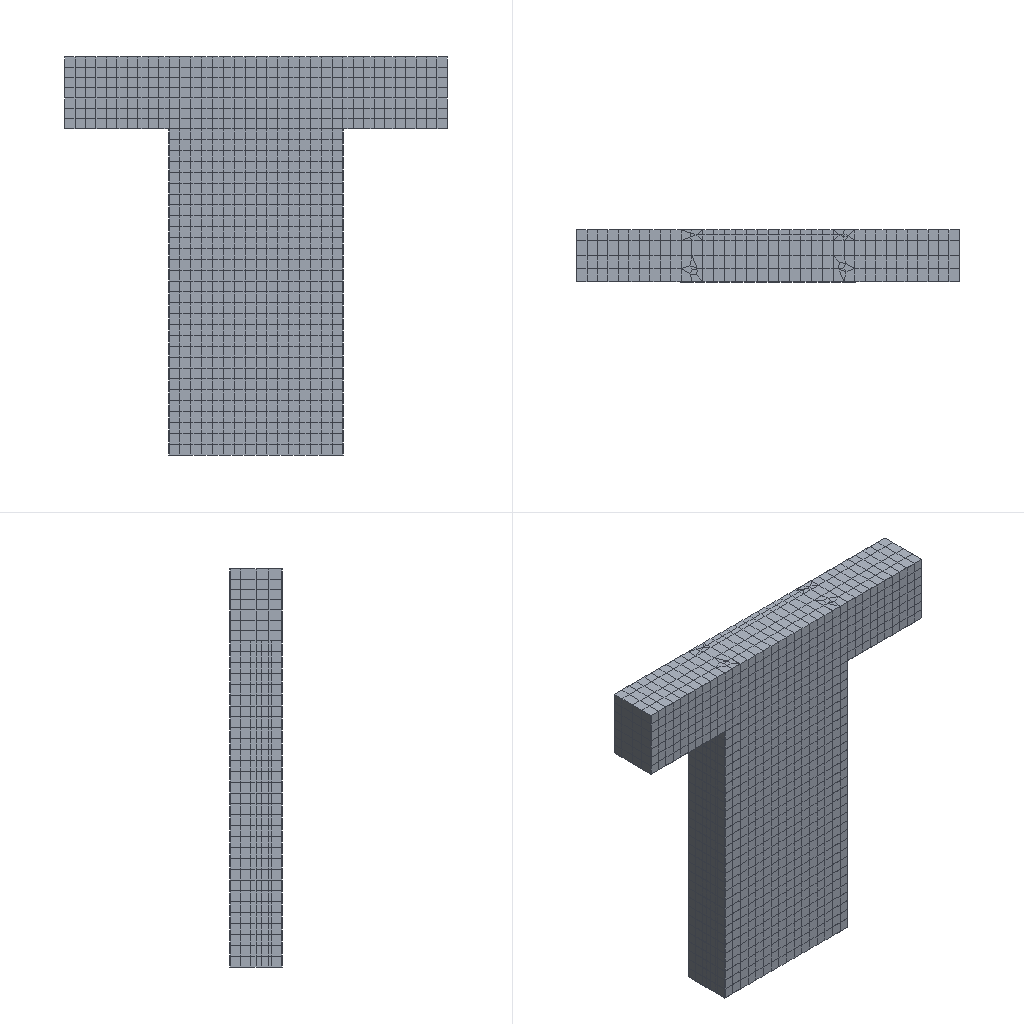Simulation study | abaqus
Set-up summary:
category,name,step,type,value,unit,region
solver,abaqus
solver,version,,,Abaqus/Standard 2020
units,not stated in the deck,,not stated
analysis,deck,,static,static
load_step,Step-1,Step-1,static
load_step,Step-2,Step-2,static
load_step,requested,,,2
mesh,nodes,,,11062
mesh,elements,,,8420
element_type,C3D6,,solid,444
element_type,R3D4,,rigid,1002
element_type,T3D2,,truss,2018
element_type,C3D8R,,solid,4956
load,load commands in deck,,count,2
bc,support commands in deck,,count,2
material,CON,,in results
material,Q235,,in results
check,setup vs results,,match,"per instance, exact: element labels, types and connectivity; labels of the nodes the elements use; coordinates of those nodes at SINGLE_PRECISION in 4 of 6 instance(s)"
Abaqus input file, long lists of numbers shortened:
*Heading
** Job name: Job-1 Model name: Model-1
** Generated by: Abaqus/CAE 2020
*Preprint, echo=NO, model=NO, history=NO, contact=NO
**
** PARTS
**
*Part, name=ban1
*Node
      1,         189.,         220.,           0.
      2,         189.,        -180.,           0.
** (494 more lines like these left out)
*Element, type=R3D4
1,  1, 13, 24,  4
2, 13, 14, 23, 24
** (499 more lines like these left out)
*Node
    497,         189.,          20.,          -5.
*Nset, nset=ban1-RefPt_, internal
497,
*Elset, elset=ban1, generate
   1,  501,    1
*End Part
**
*Part, name=ban2
*Node
      1,         189.,         220.,        1835.
      2,         189.,        -180.,        1835.
** (494 more lines like these left out)
*Element, type=R3D4
1,  1, 13, 24,  4
2, 13, 14, 23, 24
** (499 more lines like these left out)
*Node
    497,         189.,          20.,        1830.
*Nset, nset=ban2-RefPt_, internal
497,
*Elset, elset=ban2, generate
   1,  501,    1
*End Part
**
*Part, name=con
*Node
      1,         489.,          90.,        1500.
      2,        -111.,          90.,        1500.
** (5932 more lines like these left out)
*Element, type=C3D8R
  1,    5, 1585,  129,    1, 1654, 3925, 3903, 1653
  2, 1585, 1586,  130,  129, 3925, 3926, 3904, 3903
** (3814 more lines like these left out)
*Element, type=C3D6
1093,    5,   23,    1,  345,  546,  307
1094, 2438,   27,   28, 4466,  439,  547
** (442 more lines like these left out)
*Nset, nset=Set-12
    1,    2,    3,    4,    5,    6,    7,    8,    9,   10,   11,   12,   13,   14,   15,   16
   17,   18,   19,   20,   21,   22,   23,   24,   25,   26,   27,   28,   29,   30,   31,   32
** (360 more lines like these left out)
*Elset, elset=Set-12
    1,    2,    3,    4,    5,    6,    7,    8,    9,   10,   11,   12,   13,   14,   15,   16
   17,   18,   19,   20,   21,   22,   23,   24,   25,   26,   27,   28,   29,   30,   31,   32
** (249 more lines like these left out)
*Nset, nset=Set-14, generate
    1,  5934,     1
*Elset, elset=Set-14, generate
    1,  4260,     1
** Section: con
*Solid Section, elset=Set-14, material=con
,
*End Part
**
*Part, name=fiber
*Node
      1,         734.,          52.,        1525.
      2,         734.,         115.,        1525.
** (1652 more lines like these left out)
*Element, type=T3D2
1, 2, 1
2,   3, 873
** (2016 more lines like these left out)
*Nset, nset=Set-3, generate
    1,  1654,     1
*Elset, elset=Set-3, generate
    1,  2018,     1
*Nset, nset=nei
    1,    2,    3,    4,    5,    6,    7,    8,    9,   10,   11,   12,   13,   14,   15,   16
   17,   18,   19,   20,   21,   22,   23,   24,   25,   26,   27,   28,   29,   30,   31,   32
** (39 more lines like these left out)
*Elset, elset=nei
    1,    2,    3,    4,    5,    6,    7,    8,    9,   10,   11,   12,   13,   14,   15,   16
   17,   18,   19,   20,   21,   22,   23,   24,   25,   26,   27,   28,   29,   30,   31,   32
** (45 more lines like these left out)
** Section: fiber
*Solid Section, elset=Set-3, material=q235
12.56,
*End Part
**
*Part, name=liang1
*Node
      1,         588.,         140.,        1500.
      2,         588.,         140.,           0.
** (1238 more lines like these left out)
*Element, type=C3D8R
 1,   8, 145, 922, 176,   1,  57, 893, 116
 2, 145, 144, 923, 922,  57,  58, 894, 893
** (568 more lines like these left out)
*Nset, nset=Set-1, generate
    1,  1240,     1
*Elset, elset=Set-1, generate
   1,  570,    1
** Section: liang
*Solid Section, elset=Set-1, material=q235
,
*End Part
**
*Part, name=liang2
*Node
      1,        -112.,         -99.,           0.
      2,        -112.,         -99.,        1500.
** (1238 more lines like these left out)
*Element, type=C3D8R
 1, 174, 893, 922, 173,   1,  57, 114,   4
 2, 893, 894, 923, 922,  57,  58, 113, 114
** (568 more lines like these left out)
*Nset, nset=Set-1, generate
    1,  1240,     1
*Elset, elset=Set-1, generate
   1,  570,    1
** Section: liang
*Solid Section, elset=Set-1, material=q235
,
*End Part
**
**
** ASSEMBLY
**
*Assembly, name=Assembly
**
*Instance, name=ban1-1, part=ban1
*End Instance
**
*Instance, name=ban2-1, part=ban2
*End Instance
**
*Instance, name=con-1, part=con
*End Instance
**
*Instance, name=fiber-1, part=fiber
*End Instance
**
*Instance, name=liang1-1, part=liang1
*End Instance
**
*Instance, name=liang2-1, part=liang2
*End Instance
**
*Nset, nset=Set-4, instance=ban2-1
 497,
*Nset, nset=Set-5, instance=ban1-1
 497,
*Nset, nset=Set-6, instance=ban1-1
 497,
*Nset, nset=insert, instance=fiber-1
    1,    2,    3,    4,    5,    6,    7,    8,    9,   10,   11,   12,   13,   14,   15,   16
   17,   18,   19,   20,   21,   22,   23,   24,   25,   26,   27,   28,   29,   30,   31,   32
** (42 more lines like these left out)
*Nset, nset=m_Set-6, instance=fiber-1
    1,    2,    3,    4,    5,    6,    7,    8,    9,   10,   11,   12,   13,   14,   15,   16
   17,   18,   19,   20,   21,   22,   23,   24,   25,   26,   27,   28,   29,   30,   31,   32
** (40 more lines like these left out)
*Elset, elset=m_Set-6, instance=fiber-1
    1,    2,    3,    4,    5,    6,    7,    8,    9,   10,   11,   12,   13,   14,   15,   16
   17,   18,   19,   20,   21,   22,   23,   24,   25,   26,   27,   28,   29,   30,   31,   32
** (48 more lines like these left out)
*Nset, nset=m_Set-8, instance=fiber-1
    1,    2,    3,    4,    5,    6,    7,    8,    9,   10,   11,   12,   13,   14,   15,   16
   17,   18,   19,   20,   21,   22,   23,   24,   25,   26,   27,   28,   29,   30,   31,   32
** (38 more lines like these left out)
*Elset, elset=m_Set-8, instance=fiber-1
    1,    2,    3,    4,    5,    6,    7,    8,    9,   10,   11,   12,   13,   14,   15,   16
   17,   18,   19,   20,   21,   22,   23,   24,   25,   26,   27,   28,   29,   30,   31,   32
** (45 more lines like these left out)
*Nset, nset=m_Set-10, instance=fiber-1
    1,    2,    3,    4,    5,    6,    7,    8,    9,   10,   11,   12,   13,   14,   15,   16
   17,   18,   19,   20,   21,   22,   23,   24,   25,   26,   27,   28,   29,   30,   31,   32
** (38 more lines like these left out)
*Elset, elset=m_Set-10, instance=fiber-1
    1,    2,    3,    4,    5,    6,    7,    8,    9,   10,   11,   12,   13,   14,   15,   16
   17,   18,   19,   20,   21,   22,   23,   24,   25,   26,   27,   28,   29,   30,   31,   32
** (45 more lines like these left out)
*Nset, nset=m_Set-12, instance=fiber-1
    1,    2,    3,    4,    5,    6,    7,    8,    9,   10,   11,   12,   13,   14,   15,   16
   17,   18,   19,   20,   21,   22,   23,   24,   25,   26,   27,   28,   29,   30,   31,   32
** (91 more lines like these left out)
*Elset, elset=m_Set-12, instance=fiber-1
    1,    2,    3,    4,    5,    6,    7,    8,    9,   10,   11,   12,   13,   14,   15,   16
   17,   18,   19,   20,   21,   22,   23,   24,   25,   26,   27,   28,   29,   30,   31,   32
** (110 more lines like these left out)
*Nset, nset=s_Set-6, instance=con-1
    1,    2,    3,    4,    5,    6,    7,    8,    9,   10,   11,   12,   13,   14,   15,   16
   17,   18,   19,   20,   21,   22,   23,   24,   25,   26,   27,   28,   29,   30,   31,   32
** (360 more lines like these left out)
*Elset, elset=s_Set-6, instance=con-1
    1,    2,    3,    4,    5,    6,    7,    8,    9,   10,   11,   12,   13,   14,   15,   16
   17,   18,   19,   20,   21,   22,   23,   24,   25,   26,   27,   28,   29,   30,   31,   32
** (249 more lines like these left out)
*Nset, nset=s_Set-10, instance=con-1, generate
    1,  5934,     1
*Elset, elset=s_Set-10, instance=con-1, generate
    1,  4260,     1
*Nset, nset=s_Set-12, instance=con-1, generate
    1,  5934,     1
*Elset, elset=s_Set-12, instance=con-1, generate
    1,  4260,     1
*Elset, elset=_m_Surf-1_SPOS, internal, instance=ban1-1
   8,   9,  10,  11,  12,  13,  14,  15,  16,  17,  18,  19,  20,  21,  22,  23
  24,  25,  26,  27,  28,  29,  30,  31,  32,  33,  34,  35,  36,  37,  38,  39
** (12 more lines like these left out)
*Surface, type=ELEMENT, name=m_Surf-1
_m_Surf-1_SPOS, SPOS
*Elset, elset=_m_Surf-3_SPOS, internal, instance=ban2-1
 128, 129, 130, 131, 132, 133, 134, 135, 136, 137, 138, 139, 140, 141, 142, 143
 144, 145, 146, 147, 148, 149, 150, 151, 152, 153, 154, 155, 156, 157, 158, 159
** (12 more lines like these left out)
*Surface, type=ELEMENT, name=m_Surf-3
_m_Surf-3_SPOS, SPOS
*Elset, elset=_m_Surf-5_S1, internal, instance=con-1, generate
 3670,  3673,     1
*Elset, elset=_m_Surf-5_S5, internal, instance=con-1
  444,  468,  492,  516,  540,  564,  588,  612,  636,  660,  684,  708,  732,  756,  780,  804
  828,  852,  876,  900,  924,  948,  972,  996, 1020, 1044, 1068, 1092, 2104, 2164, 2200, 2208
** (4 more lines like these left out)
*Elset, elset=_m_Surf-5_S4, internal, instance=con-1
 2193, 2198, 2201, 2206, 2209, 2214, 2217, 2222, 2225, 2230, 2233, 2238, 2241, 2246, 2249, 2254
 2257, 2262, 2265, 2270, 2273, 2278, 2281, 2286, 2289, 2294, 2297, 2302, 2305, 2310, 2313, 2318
** (10 more lines like these left out)
*Elset, elset=_m_Surf-5_S3, internal, instance=con-1
 2197, 2205, 2213, 2221, 2229, 2237, 2245, 2253, 2261, 2269, 2277, 2285, 2293, 2301, 2309, 2317
 2325, 2333, 2341, 2349, 2357, 2365, 2373, 2381, 2389, 2397, 2405, 2413, 2418, 2422, 2426, 2430
** (2 more lines like these left out)
*Elset, elset=_m_Surf-5_S6, internal, instance=con-1
 1396, 1420, 1444, 1468, 1492, 1516, 1540, 1564, 1588, 1612, 1636, 1660, 1684, 1708, 1732, 1756
 1780, 1804, 1828, 1852, 1876, 1900, 1924, 1948, 1972, 1996, 2020, 2044, 2068, 2128, 2197, 2199
** (4 more lines like these left out)
*Surface, type=ELEMENT, name=m_Surf-5
_m_Surf-5_S1, S1
_m_Surf-5_S5, S5
_m_Surf-5_S4, S4
_m_Surf-5_S6, S6
_m_Surf-5_S3, S3
*Elset, elset=_m_Surf-7_S2, internal, instance=liang1-1
   1,   2,   3,   4,   5,   6,   7,   8,   9,  10,  11,  12,  13,  14,  15,  16
  17,  18,  19,  20,  21,  22,  23,  24,  25,  26,  27,  28,  29,  30,  31,  32
** (6 more lines like these left out)
*Elset, elset=_m_Surf-7_S5, internal, instance=liang1-1
 151, 152, 153, 154, 155, 156, 157, 158, 159, 160, 161, 162, 163, 164, 165, 166
 167, 168, 169, 170, 171, 172, 173, 174, 175, 176, 177, 178, 179, 180, 181, 182
** (6 more lines like these left out)
*Elset, elset=_m_Surf-7_S4, internal, instance=liang1-1
  61,  62,  63,  64,  65,  66,  67,  68,  69,  70,  71,  72,  73,  74,  75,  76
  77,  78,  79,  80,  81,  82,  83,  84,  85,  86,  87,  88,  89,  90, 270, 390
*Elset, elset=_m_Surf-7_S6, internal, instance=liang1-1
 241, 361
*Elset, elset=_m_Surf-7_S1, internal, instance=liang1-1
 241, 242, 243, 244, 245, 246, 247, 248, 249, 250, 251, 252, 253, 254, 255, 256
 257, 258, 259, 260, 261, 262, 263, 264, 265, 266, 267, 268, 269, 270, 541, 542
** (2 more lines like these left out)
*Elset, elset=_m_Surf-7_S3, internal, instance=liang1-1, generate
 361,  540,    1
*Surface, type=ELEMENT, name=m_Surf-7
_m_Surf-7_S2, S2
_m_Surf-7_S5, S5
_m_Surf-7_S4, S4
_m_Surf-7_S6, S6
_m_Surf-7_S1, S1
_m_Surf-7_S3, S3
*Elset, elset=_m_Surf-9_S6, internal, instance=con-1
 2194, 2202, 2210, 2218, 2226, 2234, 2242, 2250, 2258, 2266, 2274, 2282, 2290, 2298, 2306, 2314
 2322, 2330, 2338, 2346, 2354, 2362, 2370, 2378, 2386, 2394, 2402, 2410, 2531, 2535, 2539, 2543
** (4 more lines like these left out)
*Elset, elset=_m_Surf-9_S3, internal, instance=con-1
 2199, 2207, 2215, 2223, 2231, 2239, 2247, 2255, 2263, 2271, 2279, 2287, 2295, 2303, 2311, 2319
 2327, 2335, 2343, 2351, 2359, 2367, 2375, 2383, 2391, 2399, 2407, 2415, 2646, 2653, 2660, 2667
*Surface, type=ELEMENT, name=m_Surf-9
_m_Surf-9_S6, S6
_m_Surf-9_S3, S3
*Elset, elset=_m_Surf-11_S6, internal, instance=con-1
 2711, 2719, 2727, 2735, 2743, 2751, 2759, 2767, 2775, 2783, 2791, 2799, 2807, 2815, 2823, 2831
 2839, 2847, 2855, 2863, 2871, 2879, 2887, 2895, 2903, 2911, 2919, 2927, 2935, 2949, 2973, 2974
** (2 more lines like these left out)
*Elset, elset=_m_Surf-11_S3, internal, instance=con-1
 2709, 2717, 2725, 2733, 2741, 2749, 2757, 2765, 2773, 2781, 2789, 2797, 2805, 2813, 2821, 2829
 2837, 2845, 2853, 2861, 2869, 2877, 2885, 2893, 2901, 2909, 2917, 2925, 2933, 2940, 2947, 2954
*Elset, elset=_m_Surf-11_S4, internal, instance=con-1
 1094, 1100, 1106, 1112, 1118, 1124, 1130, 1136, 1142, 1148, 1154, 1160, 1166, 1172, 1178, 1184
 1190, 1196, 1202, 1208, 1214, 1220, 1226, 1232, 1238, 1244, 1250, 1256, 2961, 2968
*Surface, type=ELEMENT, name=m_Surf-11
_m_Surf-11_S6, S6
_m_Surf-11_S3, S3
_m_Surf-11_S4, S4
*Elset, elset=_m_Surf-14_S1, internal, instance=con-1
 3653, 3654, 3655, 3656, 3670, 3671, 3672, 3673
*Elset, elset=_m_Surf-14_S5, internal, instance=con-1
  444,  468,  492,  516,  540,  564,  588,  612,  636,  660,  684,  708,  732,  756,  780,  804
  828,  852,  876,  900,  924,  948,  972,  996, 1020, 1044, 1068, 1092, 2104, 2164, 2200, 2208
** (4 more lines like these left out)
*Elset, elset=_m_Surf-14_S4, internal, instance=con-1
 2193, 2198, 2201, 2206, 2209, 2214, 2217, 2222, 2225, 2230, 2233, 2238, 2241, 2246, 2249, 2254
 2257, 2262, 2265, 2270, 2273, 2278, 2281, 2286, 2289, 2294, 2297, 2302, 2305, 2310, 2313, 2318
** (10 more lines like these left out)
*Elset, elset=_m_Surf-14_S3, internal, instance=con-1
 2197, 2205, 2213, 2221, 2229, 2237, 2245, 2253, 2261, 2269, 2277, 2285, 2293, 2301, 2309, 2317
 2325, 2333, 2341, 2349, 2357, 2365, 2373, 2381, 2389, 2397, 2405, 2413, 2418, 2422, 2426, 2430
** (2 more lines like these left out)
*Elset, elset=_m_Surf-14_S6, internal, instance=con-1
 1396, 1420, 1444, 1468, 1492, 1516, 1540, 1564, 1588, 1612, 1636, 1660, 1684, 1708, 1732, 1756
 1780, 1804, 1828, 1852, 1876, 1900, 1924, 1948, 1972, 1996, 2020, 2044, 2068, 2128, 2197, 2199
** (4 more lines like these left out)
*Surface, type=ELEMENT, name=m_Surf-14
_m_Surf-14_S1, S1
_m_Surf-14_S5, S5
_m_Surf-14_S4, S4
_m_Surf-14_S6, S6
_m_Surf-14_S3, S3
*Elset, elset=_s_Surf-1_S2, internal, instance=con-1, generate
 361,  420,    1
*Surface, type=ELEMENT, name=s_Surf-1
_s_Surf-1_S2, S2
*Elset, elset=_s_Surf-3_S5, internal, instance=con-1
 3001, 3023, 3045, 3067, 3089, 3111, 3133, 3241, 3244, 3283, 3286, 3325, 3328, 3367, 3370, 3409
 3412, 3451, 3454, 3493, 3496, 3535, 3538, 3577, 3580, 3619, 3622, 3878, 3880, 3920, 3922, 3962
** (1 more lines like these left out)
*Elset, elset=_s_Surf-3_S3, internal, instance=con-1
 3002, 3024, 3046, 3068, 3090, 3112, 3134, 3242, 3243, 3245, 3284, 3285, 3287, 3326, 3327, 3329
 3368, 3369, 3371, 3410, 3411, 3413, 3452, 3453, 3455, 3494, 3495, 3497, 3536, 3537, 3539, 3578
** (3 more lines like these left out)
*Elset, elset=_s_Surf-3_S2, internal, instance=con-1, generate
 2105,  2164,     1
*Elset, elset=_s_Surf-3_S4, internal, instance=con-1
 3240, 3282, 3324, 3366, 3408, 3450, 3492, 3534, 3576, 3618, 3882, 3924, 3966, 4008, 4050, 4092
 4134, 4176, 4218, 4260
*Surface, type=ELEMENT, name=s_Surf-3
_s_Surf-3_S5, S5
_s_Surf-3_S3, S3
_s_Surf-3_S2, S2
_s_Surf-3_S4, S4
*Elset, elset=_s_Surf-5_S4, internal, instance=liang2-1
  30,  60,  90, 120, 181, 182, 183, 184, 185, 186, 187, 188, 189, 190, 191, 192
 193, 194, 195, 196, 197, 198, 199, 200, 201, 202, 203, 204, 205, 206, 207, 208
** (1 more lines like these left out)
*Elset, elset=_s_Surf-5_S6, internal, instance=liang2-1
  91, 151, 152, 153, 154, 155, 156, 157, 158, 159, 160, 161, 162, 163, 164, 165
 166, 167, 168, 169, 170, 171, 172, 173, 174, 175, 176, 177, 178, 179, 180, 181
** (3 more lines like these left out)
*Elset, elset=_s_Surf-5_S2, internal, instance=liang2-1
  91,  92,  93,  94,  95,  96,  97,  98,  99, 100, 101, 102, 103, 104, 105, 106
 107, 108, 109, 110, 111, 112, 113, 114, 115, 116, 117, 118, 119, 120, 151, 271
** (8 more lines like these left out)
*Elset, elset=_s_Surf-5_S3, internal, instance=liang2-1
   1,   2,   3,   4,   5,   6,   7,   8,   9,  10,  11,  12,  13,  14,  15,  16
  17,  18,  19,  20,  21,  22,  23,  24,  25,  26,  27,  28,  29,  30,  31,  32
** (4 more lines like these left out)
*Elset, elset=_s_Surf-5_S5, internal, instance=liang2-1
  91,  92,  93,  94,  95,  96,  97,  98,  99, 100, 101, 102, 103, 104, 105, 106
 107, 108, 109, 110, 111, 112, 113, 114, 115, 116, 117, 118, 119, 120, 151, 152
** (8 more lines like these left out)
*Elset, elset=_s_Surf-5_S1, internal, instance=liang2-1
  91,  92,  93,  94,  95,  96,  97,  98,  99, 100, 101, 102, 103, 104, 105, 106
 107, 108, 109, 110, 111, 112, 113, 114, 115, 116, 117, 118, 119, 120, 180, 211
** (6 more lines like these left out)
*Surface, type=ELEMENT, name=s_Surf-5
_s_Surf-5_S4, S4
_s_Surf-5_S6, S6
_s_Surf-5_S2, S2
_s_Surf-5_S3, S3
_s_Surf-5_S5, S5
_s_Surf-5_S1, S1
*Elset, elset=_s_Surf-7_S1, internal, instance=con-1, generate
 3001,  3008,     1
*Elset, elset=_s_Surf-7_S3, internal, instance=con-1
  433,  457,  481,  505,  529,  553,  577,  601,  625,  649,  673,  697,  721,  745,  769,  793
  817,  841,  865,  889,  913,  937,  961,  985, 1009, 1033, 1057, 1081, 1093, 1099, 1105, 1111
** (4 more lines like these left out)
*Elset, elset=_s_Surf-7_S4, internal, instance=con-1
 1095, 1101, 1107, 1113, 1119, 1125, 1131, 1137, 1143, 1149, 1155, 1161, 1167, 1173, 1179, 1185
 1191, 1197, 1203, 1209, 1215, 1221, 1227, 1233, 1239, 1245, 1251, 1257, 1262, 1266, 1270, 1274
** (6 more lines like these left out)
*Elset, elset=_s_Surf-7_S5, internal, instance=con-1
 1095, 1101, 1107, 1113, 1119, 1125, 1131, 1137, 1143, 1149, 1155, 1161, 1167, 1173, 1179, 1185
 1191, 1197, 1203, 1209, 1215, 1221, 1227, 1233, 1239, 1245, 1251, 1257, 1263, 1264, 1267, 1268
** (8 more lines like these left out)
*Elset, elset=_s_Surf-7_S6, internal, instance=con-1
 2707, 2713, 2715, 2721, 2723, 2729, 2731, 2737, 2739, 2745, 2747, 2753, 2755, 2761, 2763, 2769
 2771, 2777, 2779, 2785, 2787, 2793, 2795, 2801, 2803, 2809, 2811, 2817, 2819, 2825, 2827, 2833
** (2 more lines like these left out)
*Surface, type=ELEMENT, name=s_Surf-7
_s_Surf-7_S1, S1
_s_Surf-7_S3, S3
_s_Surf-7_S4, S4
_s_Surf-7_S6, S6
_s_Surf-7_S5, S5
*Elset, elset=_s_Surf-9_S3, internal, instance=liang2-1, generate
 391,  540,    1
*Surface, type=ELEMENT, name=s_Surf-9
_s_Surf-9_S3, S3
*Elset, elset=_s_Surf-11_S3, internal, instance=liang1-1, generate
 391,  540,    1
*Surface, type=ELEMENT, name=s_Surf-11
_s_Surf-11_S3, S3
*Elset, elset=_s_Surf-13_S2, internal, instance=con-1, generate
 361,  420,    1
*Elset, elset=_s_Surf-13_S2, internal, instance=liang1-1
 61,
*Elset, elset=_s_Surf-13_S4, internal, instance=liang1-1
  30,  60, 360, 420, 450, 480, 510, 540
*Elset, elset=_s_Surf-13_S4, internal, instance=liang2-1
 120, 300, 330, 390
*Elset, elset=_s_Surf-13_S1, internal, instance=liang1-1
 120, 150
*Elset, elset=_s_Surf-13_S1, internal, instance=liang2-1
 150, 180
*Elset, elset=_s_Surf-13_S6, internal, instance=liang1-1
 151, 181, 211, 241, 271, 301, 361
*Elset, elset=_s_Surf-13_S6, internal, instance=liang2-1
   1,  31,  61, 211, 241, 331, 391, 421, 451, 481, 511
*Elset, elset=_s_Surf-13_S5, internal, instance=liang1-1
 570,
*Elset, elset=_s_Surf-13_S3, internal, instance=liang2-1
 181, 541
*Surface, type=ELEMENT, name=s_Surf-13
_s_Surf-13_S2, S2
_s_Surf-13_S4, S4
_s_Surf-13_S6, S6
_s_Surf-13_S1, S1
_s_Surf-13_S5, S5
_s_Surf-13_S3, S3
*Elset, elset=_s_Surf-15_S2, internal, instance=con-1
  361,  362,  363,  364,  365,  366,  367,  368,  369,  370,  371,  372,  373,  374,  375,  376
  377,  378,  379,  380,  381,  382,  383,  384,  385,  386,  387,  388,  389,  390,  391,  392
** (6 more lines like these left out)
*Elset, elset=_s_Surf-15_S4, internal, instance=con-1
 3240, 3282, 3324, 3366, 3408, 3450, 3492, 3534, 3576, 3618, 3882, 3924, 3966, 4008, 4050, 4092
 4134, 4176, 4218, 4260
*Elset, elset=_s_Surf-15_S5, internal, instance=con-1
 3241, 3244, 3283, 3286, 3325, 3328, 3367, 3370, 3409, 3412, 3451, 3454, 3493, 3496, 3535, 3538
 3577, 3580, 3619, 3622, 3878, 3880, 3920, 3922, 3962, 3964, 4004, 4006, 4046, 4048, 4088, 4090
** (1 more lines like these left out)
*Elset, elset=_s_Surf-15_S3, internal, instance=con-1
 3242, 3243, 3245, 3284, 3285, 3287, 3326, 3327, 3329, 3368, 3369, 3371, 3410, 3411, 3413, 3452
 3453, 3455, 3494, 3495, 3497, 3536, 3537, 3539, 3578, 3579, 3581, 3620, 3621, 3623, 3877, 3879
** (2 more lines like these left out)
*Surface, type=ELEMENT, name=s_Surf-15
_s_Surf-15_S2, S2
_s_Surf-15_S4, S4
_s_Surf-15_S5, S5
_s_Surf-15_S3, S3
*Elset, elset=_s_Surf-16_S2, internal, instance=con-1
 2105, 2106, 2107, 2108, 2109, 2110, 2111, 2112, 2113, 2114, 2115, 2116, 2117, 2118, 2119, 2120
 2121, 2122, 2123, 2124, 2125, 2126, 2127, 2128, 2129, 2130, 2131, 2132, 2133, 2134, 2135, 2136
** (5 more lines like these left out)
*Elset, elset=_s_Surf-16_S2, internal, instance=liang1-1
 61,
*Elset, elset=_s_Surf-16_S4, internal, instance=liang1-1
  30,  60, 360, 420, 450, 480, 510, 540
*Elset, elset=_s_Surf-16_S4, internal, instance=liang2-1
 120, 300, 330, 390
*Elset, elset=_s_Surf-16_S1, internal, instance=liang1-1
 120, 150
*Elset, elset=_s_Surf-16_S1, internal, instance=liang2-1
 150, 180
*Elset, elset=_s_Surf-16_S6, internal, instance=liang1-1
 151, 181, 211, 241, 271, 301, 361
*Elset, elset=_s_Surf-16_S6, internal, instance=liang2-1
   1,  31,  61, 211, 241, 331, 391, 421, 451, 481, 511
*Elset, elset=_s_Surf-16_S5, internal, instance=liang1-1
 570,
*Elset, elset=_s_Surf-16_S3, internal, instance=liang2-1
 181, 541
*Surface, type=ELEMENT, name=s_Surf-16
_s_Surf-16_S2, S2
_s_Surf-16_S4, S4
_s_Surf-16_S6, S6
_s_Surf-16_S1, S1
_s_Surf-16_S5, S5
_s_Surf-16_S3, S3
*Elset, elset=_s_Surf-17_S3, internal, instance=liang2-1, generate
 391,  540,    1
*Surface, type=ELEMENT, name=s_Surf-17
_s_Surf-17_S3, S3
*Elset, elset=_s_Surf-18_S2, internal, instance=con-1
 2105, 2106, 2107, 2108, 2109, 2110, 2111, 2112, 2113, 2114, 2115, 2116, 2117, 2118, 2119, 2120
 2121, 2122, 2123, 2124, 2125, 2126, 2127, 2128, 2129, 2130, 2131, 2132, 2133, 2134, 2135, 2136
** (5 more lines like these left out)
*Elset, elset=_s_Surf-18_S2, internal, instance=liang1-1
 61,
*Elset, elset=_s_Surf-18_S4, internal, instance=liang1-1
  30,  60, 360, 420, 450, 480, 510, 540
*Elset, elset=_s_Surf-18_S4, internal, instance=liang2-1
 120, 300, 330, 390
*Elset, elset=_s_Surf-18_S1, internal, instance=liang1-1
 120, 150
*Elset, elset=_s_Surf-18_S1, internal, instance=liang2-1
 150, 180
*Elset, elset=_s_Surf-18_S6, internal, instance=liang1-1
 151, 181, 211, 241, 271, 301, 361
*Elset, elset=_s_Surf-18_S6, internal, instance=liang2-1
   1,  31,  61, 211, 241, 331, 391, 421, 451, 481, 511
*Elset, elset=_s_Surf-18_S5, internal, instance=liang1-1
 570,
*Elset, elset=_s_Surf-18_S3, internal, instance=liang2-1
 181, 541
*Surface, type=ELEMENT, name=s_Surf-18
_s_Surf-18_S2, S2
_s_Surf-18_S4, S4
_s_Surf-18_S6, S6
_s_Surf-18_S1, S1
_s_Surf-18_S5, S5
_s_Surf-18_S3, S3
*Elset, elset=_s_Surf-19_S2, internal, instance=con-1
  361,  362,  363,  364,  365,  366,  367,  368,  369,  370,  371,  372,  373,  374,  375,  376
  377,  378,  379,  380,  381,  382,  383,  384,  385,  386,  387,  388,  389,  390,  391,  392
** (6 more lines like these left out)
*Elset, elset=_s_Surf-19_S4, internal, instance=con-1
 3240, 3282, 3324, 3366, 3408, 3450, 3492, 3534, 3576, 3618, 3882, 3924, 3966, 4008, 4050, 4092
 4134, 4176, 4218, 4260
*Elset, elset=_s_Surf-19_S5, internal, instance=con-1
 3241, 3244, 3283, 3286, 3325, 3328, 3367, 3370, 3409, 3412, 3451, 3454, 3493, 3496, 3535, 3538
 3577, 3580, 3619, 3622, 3878, 3880, 3920, 3922, 3962, 3964, 4004, 4006, 4046, 4048, 4088, 4090
** (1 more lines like these left out)
*Elset, elset=_s_Surf-19_S3, internal, instance=con-1
 3242, 3243, 3245, 3284, 3285, 3287, 3326, 3327, 3329, 3368, 3369, 3371, 3410, 3411, 3413, 3452
 3453, 3455, 3494, 3495, 3497, 3536, 3537, 3539, 3578, 3579, 3581, 3620, 3621, 3623, 3877, 3879
** (2 more lines like these left out)
*Surface, type=ELEMENT, name=s_Surf-19
_s_Surf-19_S2, S2
_s_Surf-19_S4, S4
_s_Surf-19_S5, S5
_s_Surf-19_S3, S3
*Rigid Body, ref node=ban1-1.ban1-RefPt_, elset=ban1-1.ban1
*Rigid Body, ref node=ban2-1.ban2-RefPt_, elset=ban2-1.ban2
** Constraint: Constraint-4
*Tie, name=Constraint-4, adjust=yes
s_Surf-11, m_Surf-11
** Constraint: Constraint-ban1
*Tie, name=Constraint-ban1, adjust=yes
s_Surf-18, m_Surf-1
** Constraint: Constraint-ban2
*Tie, name=Constraint-ban2, adjust=yes
s_Surf-19, m_Surf-3
** Constraint: Constraint-liang
*Tie, name=Constraint-liang, adjust=yes
m_Surf-9, s_Surf-17
** Constraint: Constraint-nei
*Embedded Element, host elset=s_Set-12
m_Set-12
*End Assembly
*Amplitude, name=Amp-1
             0.,              0.,              1.,              1.
*Amplitude, name=Amp-load
             0.,              0.,             0.5,             0.1,              1.,            -0.1,             1.5,              0.
             2.,             0.4,             2.5,            -0.4,              3.,              0.,             3.5,             0.6
             4.,            -0.6,             4.5,              0.,              5.,             0.9,             5.5,            -0.9
             6.,              0.,             6.5,              1.,              7.,             -1.,             7.5,              0.
             8.,             1.3,             8.5,            -1.3,              9.,              0.,             9.5,             1.6
            10.,            -1.6,            10.5,              0.,             11.,             1.9,            11.5,            -1.9
            12.,              0.,            12.5,             2.4,             13.,            -2.4,            13.5,              0.
            14.,             2.8,            14.5,            -2.8,             15.,              0.,            15.5,             3.2
            16.,            -3.2,            16.5,              0.,             17.,             3.6,            17.5,            -3.6
            18.,              0.,            18.5,              4.,             19.,             -4.,            19.5,              0.
            20.,             4.4,            20.5,            -4.4,             21.,              0.,            21.5,             4.8
            22.,            -4.8,            22.5,              0.,             23.,             5.2,            23.5,            -5.2
            24.,              0.,            24.5,             5.6,             25.,            -5.6,            25.5,              0.
            26.,              6.,            26.5,             -6.,             27.,              0.,            27.5,             6.5
            28.,            -6.5,            28.5,              0.,             29.,              7.,            29.5,             -7.
            30.,              0.,            30.5,             7.5,             31.,            -7.5,            31.5,              0.
            32.,              8.,            32.5,             -8.,             33.,              0.,            33.5,             8.5
            34.,            -8.5,            34.5,              0.,             35.,              9.,            35.5,             -9.
            36.,              0.,            36.5,             9.6,             37.,            -9.6,            37.5,              0.
            38.,            10.2,            38.5,           -10.2,             39.,              0.,            39.5,            10.8
            40.,           -10.8,            40.5,              0.,             41.,            11.4,            41.5,           -11.4
            42.,              0.,            42.5,             12.,             43.,            -12.,            43.5,              0.
            44.,            12.7,            44.5,           -12.7,             45.,              0.,            45.5,            13.4
            46.,           -13.4,            46.5,              0.,             47.,            14.1,            47.5,           -14.1
            48.,              0.,            48.5,            14.9,             49.,           -14.9,            49.5,              0.
            50.,            15.7,            50.5,           -15.7,             51.,              0.,            51.5,            16.5
            52.,           -16.5,            52.5,              0.
**
** MATERIALS
**
*Material, name=con
*Elastic
2260., 0.2
*Concrete Damaged Plasticity
45.,     0.1,    1.16,  0.6667, 0.00075
*Concrete Compression Hardening
  2.669,         0.
  3.127, 0.001499
  3.503, 0.001799
 3.659, 0.001949
  3.795, 0.002099
 3.909, 0.002249
  4.003, 0.002399
 4.076,  0.002549
  4.128, 0.002699
 4.16, 0.002849
    4.17, 0.002999
  1.087,  0.003299
   0.532, 0.003599
  0.1198, 0.003899
  0.0364, 0.004199
   0.013, 0.004499
    0.01, 0.004799
*Concrete Tension Stiffening
   0.1984,         0.
   0.2325, 0.0015
   0.2604, 0.0018
 0.272, 0.00195
   0.2821, 0.0021
 0.2906, 0.00225
   0.2976, 0.0024
 0.303, 0.00255
   0.3069, 0.0027
 0.3092, 0.00285
     0.31, 0.003
   0.3038, 0.0033
   0.2976, 0.0036
   0.2914, 0.0039
   0.2852, 0.0042
    0.279, 0.0045
   0.2728, 0.0048
*Concrete Compression Damage
        0.,         0.
 0.0395, 0.001499
 0.07207, 0.001799
 0.08879, 0.001949
   0.1058, 0.002099
  0.1232, 0.002249
    0.1409, 0.002399
  0.159,  0.002549
  0.1775, 0.002699
  0.1964, 0.002849
  0.2158, 0.002999
  0.2598,  0.003299
  0.2985, 0.003599
  0.3331, 0.003899
  0.3643, 0.004199
  0.3925, 0.004499
  0.4184, 0.004799
      0.43,    0.00485
      0.45,     0.0051
       0.5,     0.0054
      0.55,      0.006
       0.6,     0.0063
      0.63,     0.0066
      0.67,     0.0069
       0.7,     0.0072
      0.74,     0.0075
      0.78,     0.0079
      0.82,     0.0081
      0.88,     0.0085
      0.95,      0.009
*Concrete Tension Damage
       0.,         0.
 0.7381, 0.0015
 0.747, 0.0018
 0.7516, 0.00195
 0.7562, 0.0021
 0.7609, 0.00225
 0.7658, 0.0024
 0.7707, 0.00255
 0.7757, 0.0027
 0.7809, 0.00285
 0.7862, 0.003
 0.7982, 0.0033
 0.8087, 0.0036
 0.8182, 0.0039
 0.8267, 0.0042
 0.8344, 0.0045
  0.8414, 0.0048
*Material, name=q235
*Elastic
154500., 0.25
*Plastic
 140.754,         0.
 247.869, 0.002268
 289.318, 0.004368
    300.,      0.005
    250.,     0.0053
    200.,      0.006
    150.,      0.008
     90.,      0.009
     40.,       0.01
     10.,       0.02
**
** INTERACTION PROPERTIES
**
*Surface Interaction, name=IntProp-1
1.,
*Friction, slip tolerance=0.005
 0.2,
*Surface Behavior, pressure-overclosure=HARD
**
** INTERACTIONS
**
** Interaction: Int-1
*Contact Pair, interaction=IntProp-1, type=SURFACE TO SURFACE
m_Surf-14, s_Surf-5
** Interaction: Int-2
*Contact Pair, interaction=IntProp-1, type=SURFACE TO SURFACE
s_Surf-7, m_Surf-7
** ----------------------------------------------------------------
**
** STEP: Step-1
**
*Step, name=Step-1, nlgeom=NO, inc=1000
*Static
0.01, 1., 1e-05, 1.
**
** BOUNDARY CONDITIONS
**
** Name: [REDACTED] : Symmetric / antisymmetric / fully fixed
*Boundary
Set-4, ENCASTRE
**
** LOADS
**
** Name: Load   Type: Concentrated force
*Cload, amplitude=Amp-1
Set-5, 3, 259200.
**
** OUTPUT REQUESTS
**
*Restart, write, frequency=0
**
** FIELD OUTPUT: F-Output-1
**
*Output, field, variable=PRESELECT
*Output, history, frequency=0
*End Step
** ----------------------------------------------------------------
**
** STEP: Step-2
**
*Step, name=Step-2, nlgeom=NO, inc=5000
*Static
0.1, 40., 0.0004, 40.
**
** BOUNDARY CONDITIONS
**
** Name: [REDACTED] : Displacement/rotation angle
*Boundary, amplitude=Amp-load
Set-6, 1, 1, 1.
**
** OUTPUT REQUESTS
**
*Restart, write, frequency=0
**
** FIELD OUTPUT: F-Output-1
**
*Output, field
*Node Output
CF, RF, RM, RT, U, V
*Element Output, directions=YES
DAMAGEC, DAMAGET, E, LE, MISES, MISESMAX, MISESONLY, P, PE, PEEQ, PEEQMAX, PEEQT, PEMAG, S, SDEG, SF
SSAVG
*Contact Output
CDISP, CSTRESS
**
** HISTORY OUTPUT: H-Output-1
**
*Output, history
*Node Output, nset=Set-6
RF1, U1
*End Step
Results summary:
result,step,,completed,increments=11 time=1.0/1.0
result,step,,partial,increments=163 time=14.835/40.0
result,analysis,,,static
result,last_loadstep,,,2
result,primary field,,,U
result,reaction total,,FX,0.0,model units
result,reaction total,,FY,0.0,model units
result,reaction total,,FZ,-259200.0,model units